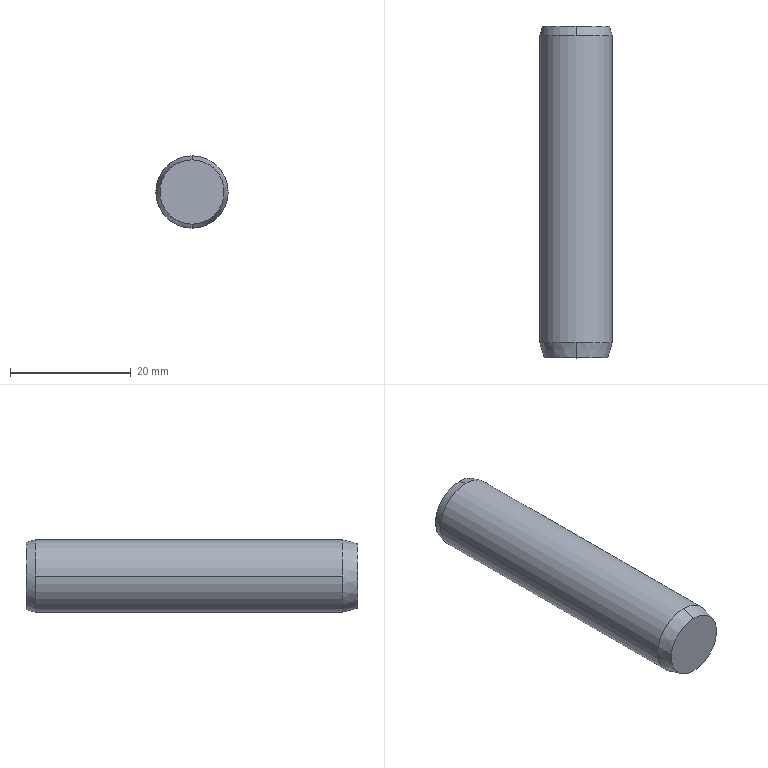Part | STEP file | 1 solid | 16 faces | box 12 x 55 x 12 mm | volume 5770 mm3 | cone 8 | cylinder 6 | plane 2 | commonest cylinder face diameters 4.917 x2 6.4 x2 12 x2
STEP:
#1=CARTESIAN_POINT('',(0.,-55.,5.33));
#2=VERTEX_POINT('',#1);
#3=CARTESIAN_POINT('',(0.,-55.,-5.33));
#4=VERTEX_POINT('',#3);
#5=CARTESIAN_POINT('',(0.,-55.,0.));
#6=DIRECTION('',(0.,1.,0.));
#7=DIRECTION('',(0.,0.,1.));
#8=AXIS2_PLACEMENT_3D('',#5,#6,#7);
#9=CIRCLE('',#8,5.33);
#10=EDGE_CURVE('',#2,#4,#9,.T.);
#11=ORIENTED_EDGE('',*,*,#10,.T.);
#12=CARTESIAN_POINT('',(0.,-52.5,-6.));
#13=VERTEX_POINT('',#12);
#14=CARTESIAN_POINT('',(0.,-55.,-5.33));
#15=DIRECTION('',(0.,0.9659,-0.2588));
#16=VECTOR('',#15,1000.);
#17=LINE('',#14,#16);
#18=EDGE_CURVE('',#4,#13,#17,.T.);
#19=ORIENTED_EDGE('',*,*,#18,.T.);
#20=CARTESIAN_POINT('',(6.,-52.5,0.));
#21=VERTEX_POINT('',#20);
#22=CARTESIAN_POINT('',(0.,-52.5,0.));
#23=DIRECTION('',(0.,1.,0.));
#24=DIRECTION('',(0.,0.,1.));
#25=AXIS2_PLACEMENT_3D('',#22,#23,#24);
#26=CIRCLE('',#25,6.);
#27=EDGE_CURVE('',#21,#13,#26,.T.);
#28=ORIENTED_EDGE('',*,*,#27,.F.);
#29=CARTESIAN_POINT('',(0.,-52.5,6.));
#30=VERTEX_POINT('',#29);
#31=CARTESIAN_POINT('',(0.,-52.5,0.));
#32=DIRECTION('',(0.,1.,0.));
#33=DIRECTION('',(0.,0.,1.));
#34=AXIS2_PLACEMENT_3D('',#31,#32,#33);
#35=CIRCLE('',#34,6.);
#36=EDGE_CURVE('',#30,#21,#35,.T.);
#37=ORIENTED_EDGE('',*,*,#36,.F.);
#38=CARTESIAN_POINT('',(0.,-55.,5.33));
#39=DIRECTION('',(0.,0.9659,0.2588));
#40=VECTOR('',#39,1000.);
#41=LINE('',#38,#40);
#42=EDGE_CURVE('',#2,#30,#41,.T.);
#43=ORIENTED_EDGE('',*,*,#42,.F.);
#44=EDGE_LOOP('',(#11,#19,#28,#37,#43));
#45=FACE_OUTER_BOUND('',#44,.T.);
#46=CARTESIAN_POINT('',(0.,-55.,0.));
#47=DIRECTION('',(0.,1.,0.));
#48=DIRECTION('',(0.,0.,1.));
#49=AXIS2_PLACEMENT_3D('',#46,#47,#48);
#50=CONICAL_SURFACE('',#49,5.33,0.2618);
#51=ADVANCED_FACE('',(#45),#50,.T.);
#52=CARTESIAN_POINT('',(-6.,-52.5,0.));
#53=VERTEX_POINT('',#52);
#54=CARTESIAN_POINT('',(0.,-52.5,0.));
#55=DIRECTION('',(0.,1.,0.));
#56=DIRECTION('',(0.,0.,1.));
#57=AXIS2_PLACEMENT_3D('',#54,#55,#56);
#58=CIRCLE('',#57,6.);
#59=EDGE_CURVE('',#53,#30,#58,.T.);
#60=ORIENTED_EDGE('',*,*,#59,.T.);
#61=ORIENTED_EDGE('',*,*,#36,.T.);
#62=CARTESIAN_POINT('',(6.,-1.6,0.));
#63=VERTEX_POINT('',#62);
#64=CARTESIAN_POINT('',(6.,-21.42,0.));
#65=DIRECTION('',(0.,1.,0.));
#66=VECTOR('',#65,1000.);
#67=LINE('',#64,#66);
#68=EDGE_CURVE('',#21,#63,#67,.T.);
#69=ORIENTED_EDGE('',*,*,#68,.T.);
#70=CARTESIAN_POINT('',(0.,-1.6,6.));
#71=VERTEX_POINT('',#70);
#72=CARTESIAN_POINT('',(0.,-1.6,0.));
#73=DIRECTION('',(0.,1.,0.));
#74=DIRECTION('',(0.,0.,1.));
#75=AXIS2_PLACEMENT_3D('',#72,#73,#74);
#76=CIRCLE('',#75,6.);
#77=EDGE_CURVE('',#71,#63,#76,.T.);
#78=ORIENTED_EDGE('',*,*,#77,.F.);
#79=CARTESIAN_POINT('',(-6.,-1.6,0.));
#80=VERTEX_POINT('',#79);
#81=CARTESIAN_POINT('',(0.,-1.6,0.));
#82=DIRECTION('',(0.,1.,0.));
#83=DIRECTION('',(0.,0.,1.));
#84=AXIS2_PLACEMENT_3D('',#81,#82,#83);
#85=CIRCLE('',#84,6.);
#86=EDGE_CURVE('',#80,#71,#85,.T.);
#87=ORIENTED_EDGE('',*,*,#86,.F.);
#88=CARTESIAN_POINT('',(-6.,-21.42,0.));
#89=DIRECTION('',(0.,1.,0.));
#90=VECTOR('',#89,1000.);
#91=LINE('',#88,#90);
#92=EDGE_CURVE('',#53,#80,#91,.T.);
#93=ORIENTED_EDGE('',*,*,#92,.F.);
#94=EDGE_LOOP('',(#60,#61,#69,#78,#87,#93));
#95=FACE_OUTER_BOUND('',#94,.T.);
#96=CARTESIAN_POINT('',(0.,-21.42,0.));
#97=DIRECTION('',(0.,1.,0.));
#98=DIRECTION('',(-1.,0.,0.));
#99=AXIS2_PLACEMENT_3D('',#96,#97,#98);
#100=CYLINDRICAL_SURFACE('',#99,6.);
#101=ADVANCED_FACE('',(#95),#100,.T.);
#102=CARTESIAN_POINT('',(0.,0.,5.571));
#103=VERTEX_POINT('',#102);
#104=CARTESIAN_POINT('',(0.,0.,-5.571));
#105=VERTEX_POINT('',#104);
#106=CARTESIAN_POINT('',(0.,0.,0.));
#107=DIRECTION('',(0.,1.,0.));
#108=DIRECTION('',(0.,0.,1.));
#109=AXIS2_PLACEMENT_3D('',#106,#107,#108);
#110=CIRCLE('',#109,5.571);
#111=EDGE_CURVE('',#103,#105,#110,.T.);
#112=ORIENTED_EDGE('',*,*,#111,.F.);
#113=CARTESIAN_POINT('',(0.,-1.6,6.));
#114=DIRECTION('',(0.,-0.9659,0.2588));
#115=VECTOR('',#114,1000.);
#116=LINE('',#113,#115);
#117=EDGE_CURVE('',#103,#71,#116,.T.);
#118=ORIENTED_EDGE('',*,*,#117,.T.);
#119=ORIENTED_EDGE('',*,*,#77,.T.);
#120=CARTESIAN_POINT('',(0.,-1.6,-6.));
#121=VERTEX_POINT('',#120);
#122=CARTESIAN_POINT('',(0.,-1.6,0.));
#123=DIRECTION('',(0.,1.,0.));
#124=DIRECTION('',(0.,0.,1.));
#125=AXIS2_PLACEMENT_3D('',#122,#123,#124);
#126=CIRCLE('',#125,6.);
#127=EDGE_CURVE('',#63,#121,#126,.T.);
#128=ORIENTED_EDGE('',*,*,#127,.T.);
#129=CARTESIAN_POINT('',(0.,-1.6,-6.));
#130=DIRECTION('',(0.,-0.9659,-0.2588));
#131=VECTOR('',#130,1000.);
#132=LINE('',#129,#131);
#133=EDGE_CURVE('',#105,#121,#132,.T.);
#134=ORIENTED_EDGE('',*,*,#133,.F.);
#135=EDGE_LOOP('',(#112,#118,#119,#128,#134));
#136=FACE_OUTER_BOUND('',#135,.T.);
#137=CARTESIAN_POINT('',(0.,-1.6,0.));
#138=DIRECTION('',(0.,-1.,0.));
#139=DIRECTION('',(0.,0.,-1.));
#140=AXIS2_PLACEMENT_3D('',#137,#138,#139);
#141=CONICAL_SURFACE('',#140,6.,0.2618);
#142=ADVANCED_FACE('',(#136),#141,.T.);
#143=CARTESIAN_POINT('',(0.,-21.42,0.));
#144=VERTEX_POINT('',#143);
#145=CARTESIAN_POINT('',(-2.459,-20.,0.));
#146=VERTEX_POINT('',#145);
#147=CARTESIAN_POINT('',(-2.459,-20.,0.));
#148=DIRECTION('',(-0.866,0.5,0.));
#149=VECTOR('',#148,1000.);
#150=LINE('',#147,#149);
#151=EDGE_CURVE('',#144,#146,#150,.T.);
#152=ORIENTED_EDGE('',*,*,#151,.F.);
#153=CARTESIAN_POINT('',(2.459,-20.,0.));
#154=VERTEX_POINT('',#153);
#155=CARTESIAN_POINT('',(2.459,-20.,0.));
#156=DIRECTION('',(0.866,0.5,0.));
#157=VECTOR('',#156,1000.);
#158=LINE('',#155,#157);
#159=EDGE_CURVE('',#144,#154,#158,.T.);
#160=ORIENTED_EDGE('',*,*,#159,.T.);
#161=CARTESIAN_POINT('',(0.,-20.,0.));
#162=DIRECTION('',(0.,1.,0.));
#163=DIRECTION('',(-1.,0.,0.));
#164=AXIS2_PLACEMENT_3D('',#161,#162,#163);
#165=CIRCLE('',#164,2.459);
#166=EDGE_CURVE('',#154,#146,#165,.T.);
#167=ORIENTED_EDGE('',*,*,#166,.T.);
#168=EDGE_LOOP('',(#152,#160,#167));
#169=FACE_OUTER_BOUND('',#168,.T.);
#170=CARTESIAN_POINT('',(0.,-20.,0.));
#171=DIRECTION('',(0.,1.,0.));
#172=DIRECTION('',(-1.,0.,0.));
#173=AXIS2_PLACEMENT_3D('',#170,#171,#172);
#174=CONICAL_SURFACE('',#173,2.459,1.047);
#175=ADVANCED_FACE('',(#169),#174,.F.);
#176=ORIENTED_EDGE('',*,*,#166,.F.);
#177=CARTESIAN_POINT('',(2.459,-1.628,0.));
#178=VERTEX_POINT('',#177);
#179=CARTESIAN_POINT('',(2.459,-21.42,0.));
#180=DIRECTION('',(0.,1.,0.));
#181=VECTOR('',#180,1000.);
#182=LINE('',#179,#181);
#183=EDGE_CURVE('',#154,#178,#182,.T.);
#184=ORIENTED_EDGE('',*,*,#183,.T.);
#185=CARTESIAN_POINT('',(-2.459,-1.628,0.));
#186=VERTEX_POINT('',#185);
#187=CARTESIAN_POINT('',(0.,-1.628,0.));
#188=DIRECTION('',(0.,1.,0.));
#189=DIRECTION('',(-1.,0.,0.));
#190=AXIS2_PLACEMENT_3D('',#187,#188,#189);
#191=CIRCLE('',#190,2.459);
#192=EDGE_CURVE('',#178,#186,#191,.T.);
#193=ORIENTED_EDGE('',*,*,#192,.T.);
#194=CARTESIAN_POINT('',(-2.459,-21.42,0.));
#195=DIRECTION('',(0.,1.,0.));
#196=VECTOR('',#195,1000.);
#197=LINE('',#194,#196);
#198=EDGE_CURVE('',#146,#186,#197,.T.);
#199=ORIENTED_EDGE('',*,*,#198,.F.);
#200=EDGE_LOOP('',(#176,#184,#193,#199));
#201=FACE_OUTER_BOUND('',#200,.T.);
#202=CARTESIAN_POINT('',(0.,-21.42,0.));
#203=DIRECTION('',(0.,1.,0.));
#204=DIRECTION('',(-1.,0.,0.));
#205=AXIS2_PLACEMENT_3D('',#202,#203,#204);
#206=CYLINDRICAL_SURFACE('',#205,2.459);
#207=ADVANCED_FACE('',(#201),#206,.F.);
#208=ORIENTED_EDGE('',*,*,#192,.F.);
#209=CARTESIAN_POINT('',(3.2,-1.2,0.));
#210=VERTEX_POINT('',#209);
#211=CARTESIAN_POINT('',(3.2,-1.2,0.));
#212=DIRECTION('',(0.866,0.5,0.));
#213=VECTOR('',#212,1000.);
#214=LINE('',#211,#213);
#215=EDGE_CURVE('',#178,#210,#214,.T.);
#216=ORIENTED_EDGE('',*,*,#215,.T.);
#217=CARTESIAN_POINT('',(-3.2,-1.2,0.));
#218=VERTEX_POINT('',#217);
#219=CARTESIAN_POINT('',(0.,-1.2,0.));
#220=DIRECTION('',(0.,1.,0.));
#221=DIRECTION('',(-1.,0.,0.));
#222=AXIS2_PLACEMENT_3D('',#219,#220,#221);
#223=CIRCLE('',#222,3.2);
#224=EDGE_CURVE('',#210,#218,#223,.T.);
#225=ORIENTED_EDGE('',*,*,#224,.T.);
#226=CARTESIAN_POINT('',(-3.2,-1.2,0.));
#227=DIRECTION('',(-0.866,0.5,0.));
#228=VECTOR('',#227,1000.);
#229=LINE('',#226,#228);
#230=EDGE_CURVE('',#186,#218,#229,.T.);
#231=ORIENTED_EDGE('',*,*,#230,.F.);
#232=EDGE_LOOP('',(#208,#216,#225,#231));
#233=FACE_OUTER_BOUND('',#232,.T.);
#234=CARTESIAN_POINT('',(0.,-1.2,0.));
#235=DIRECTION('',(0.,1.,0.));
#236=DIRECTION('',(-1.,0.,0.));
#237=AXIS2_PLACEMENT_3D('',#234,#235,#236);
#238=CONICAL_SURFACE('',#237,3.2,1.047);
#239=ADVANCED_FACE('',(#233),#238,.F.);
#240=ORIENTED_EDGE('',*,*,#224,.F.);
#241=CARTESIAN_POINT('',(3.2,0.,0.));
#242=VERTEX_POINT('',#241);
#243=CARTESIAN_POINT('',(3.2,-21.42,0.));
#244=DIRECTION('',(0.,1.,0.));
#245=VECTOR('',#244,1000.);
#246=LINE('',#243,#245);
#247=EDGE_CURVE('',#210,#242,#246,.T.);
#248=ORIENTED_EDGE('',*,*,#247,.T.);
#249=CARTESIAN_POINT('',(-3.2,0.,0.));
#250=VERTEX_POINT('',#249);
#251=CARTESIAN_POINT('',(0.,0.,0.));
#252=DIRECTION('',(0.,1.,0.));
#253=DIRECTION('',(-1.,0.,0.));
#254=AXIS2_PLACEMENT_3D('',#251,#252,#253);
#255=CIRCLE('',#254,3.2);
#256=EDGE_CURVE('',#242,#250,#255,.T.);
#257=ORIENTED_EDGE('',*,*,#256,.T.);
#258=CARTESIAN_POINT('',(-3.2,-21.42,0.));
#259=DIRECTION('',(0.,1.,0.));
#260=VECTOR('',#259,1000.);
#261=LINE('',#258,#260);
#262=EDGE_CURVE('',#218,#250,#261,.T.);
#263=ORIENTED_EDGE('',*,*,#262,.F.);
#264=EDGE_LOOP('',(#240,#248,#257,#263));
#265=FACE_OUTER_BOUND('',#264,.T.);
#266=CARTESIAN_POINT('',(0.,-21.42,0.));
#267=DIRECTION('',(0.,1.,0.));
#268=DIRECTION('',(-1.,0.,0.));
#269=AXIS2_PLACEMENT_3D('',#266,#267,#268);
#270=CYLINDRICAL_SURFACE('',#269,3.2);
#271=ADVANCED_FACE('',(#265),#270,.F.);
#272=CARTESIAN_POINT('',(0.,0.,0.));
#273=DIRECTION('',(0.,1.,0.));
#274=DIRECTION('',(-1.,0.,0.));
#275=AXIS2_PLACEMENT_3D('',#272,#273,#274);
#276=CIRCLE('',#275,3.2);
#277=EDGE_CURVE('',#250,#242,#276,.T.);
#278=ORIENTED_EDGE('',*,*,#277,.F.);
#279=ORIENTED_EDGE('',*,*,#256,.F.);
#280=EDGE_LOOP('',(#278,#279));
#281=FACE_BOUND('',#280,.T.);
#282=CARTESIAN_POINT('',(0.,0.,0.));
#283=DIRECTION('',(0.,1.,0.));
#284=DIRECTION('',(0.,0.,1.));
#285=AXIS2_PLACEMENT_3D('',#282,#283,#284);
#286=CIRCLE('',#285,5.571);
#287=EDGE_CURVE('',#105,#103,#286,.T.);
#288=ORIENTED_EDGE('',*,*,#287,.T.);
#289=ORIENTED_EDGE('',*,*,#111,.T.);
#290=EDGE_LOOP('',(#288,#289));
#291=FACE_OUTER_BOUND('',#290,.T.);
#292=CARTESIAN_POINT('',(6.,0.,0.));
#293=DIRECTION('',(0.,-1.,0.));
#294=DIRECTION('',(1.,0.,0.));
#295=AXIS2_PLACEMENT_3D('',#292,#293,#294);
#296=PLANE('',#295);
#297=ADVANCED_FACE('',(#281,#291),#296,.F.);
#298=ORIENTED_EDGE('',*,*,#247,.F.);
#299=CARTESIAN_POINT('',(0.,-1.2,0.));
#300=DIRECTION('',(0.,1.,0.));
#301=DIRECTION('',(-1.,0.,0.));
#302=AXIS2_PLACEMENT_3D('',#299,#300,#301);
#303=CIRCLE('',#302,3.2);
#304=EDGE_CURVE('',#218,#210,#303,.T.);
#305=ORIENTED_EDGE('',*,*,#304,.F.);
#306=ORIENTED_EDGE('',*,*,#262,.T.);
#307=ORIENTED_EDGE('',*,*,#277,.T.);
#308=EDGE_LOOP('',(#298,#305,#306,#307));
#309=FACE_OUTER_BOUND('',#308,.T.);
#310=CARTESIAN_POINT('',(0.,-21.42,0.));
#311=DIRECTION('',(0.,1.,0.));
#312=DIRECTION('',(-1.,0.,0.));
#313=AXIS2_PLACEMENT_3D('',#310,#311,#312);
#314=CYLINDRICAL_SURFACE('',#313,3.2);
#315=ADVANCED_FACE('',(#309),#314,.F.);
#316=ORIENTED_EDGE('',*,*,#215,.F.);
#317=CARTESIAN_POINT('',(0.,-1.628,0.));
#318=DIRECTION('',(0.,1.,0.));
#319=DIRECTION('',(-1.,0.,0.));
#320=AXIS2_PLACEMENT_3D('',#317,#318,#319);
#321=CIRCLE('',#320,2.459);
#322=EDGE_CURVE('',#186,#178,#321,.T.);
#323=ORIENTED_EDGE('',*,*,#322,.F.);
#324=ORIENTED_EDGE('',*,*,#230,.T.);
#325=ORIENTED_EDGE('',*,*,#304,.T.);
#326=EDGE_LOOP('',(#316,#323,#324,#325));
#327=FACE_OUTER_BOUND('',#326,.T.);
#328=CARTESIAN_POINT('',(0.,-1.2,0.));
#329=DIRECTION('',(0.,1.,0.));
#330=DIRECTION('',(-1.,0.,0.));
#331=AXIS2_PLACEMENT_3D('',#328,#329,#330);
#332=CONICAL_SURFACE('',#331,3.2,1.047);
#333=ADVANCED_FACE('',(#327),#332,.F.);
#334=ORIENTED_EDGE('',*,*,#183,.F.);
#335=CARTESIAN_POINT('',(0.,-20.,0.));
#336=DIRECTION('',(0.,1.,0.));
#337=DIRECTION('',(-1.,0.,0.));
#338=AXIS2_PLACEMENT_3D('',#335,#336,#337);
#339=CIRCLE('',#338,2.459);
#340=EDGE_CURVE('',#146,#154,#339,.T.);
#341=ORIENTED_EDGE('',*,*,#340,.F.);
#342=ORIENTED_EDGE('',*,*,#198,.T.);
#343=ORIENTED_EDGE('',*,*,#322,.T.);
#344=EDGE_LOOP('',(#334,#341,#342,#343));
#345=FACE_OUTER_BOUND('',#344,.T.);
#346=CARTESIAN_POINT('',(0.,-21.42,0.));
#347=DIRECTION('',(0.,1.,0.));
#348=DIRECTION('',(-1.,0.,0.));
#349=AXIS2_PLACEMENT_3D('',#346,#347,#348);
#350=CYLINDRICAL_SURFACE('',#349,2.459);
#351=ADVANCED_FACE('',(#345),#350,.F.);
#352=ORIENTED_EDGE('',*,*,#159,.F.);
#353=ORIENTED_EDGE('',*,*,#151,.T.);
#354=ORIENTED_EDGE('',*,*,#340,.T.);
#355=EDGE_LOOP('',(#352,#353,#354));
#356=FACE_OUTER_BOUND('',#355,.T.);
#357=CARTESIAN_POINT('',(0.,-20.,0.));
#358=DIRECTION('',(0.,1.,0.));
#359=DIRECTION('',(-1.,0.,0.));
#360=AXIS2_PLACEMENT_3D('',#357,#358,#359);
#361=CONICAL_SURFACE('',#360,2.459,1.047);
#362=ADVANCED_FACE('',(#356),#361,.F.);
#363=ORIENTED_EDGE('',*,*,#117,.F.);
#364=ORIENTED_EDGE('',*,*,#287,.F.);
#365=ORIENTED_EDGE('',*,*,#133,.T.);
#366=CARTESIAN_POINT('',(0.,-1.6,0.));
#367=DIRECTION('',(0.,1.,0.));
#368=DIRECTION('',(0.,0.,1.));
#369=AXIS2_PLACEMENT_3D('',#366,#367,#368);
#370=CIRCLE('',#369,6.);
#371=EDGE_CURVE('',#121,#80,#370,.T.);
#372=ORIENTED_EDGE('',*,*,#371,.T.);
#373=ORIENTED_EDGE('',*,*,#86,.T.);
#374=EDGE_LOOP('',(#363,#364,#365,#372,#373));
#375=FACE_OUTER_BOUND('',#374,.T.);
#376=CARTESIAN_POINT('',(0.,-1.6,0.));
#377=DIRECTION('',(0.,-1.,0.));
#378=DIRECTION('',(0.,0.,-1.));
#379=AXIS2_PLACEMENT_3D('',#376,#377,#378);
#380=CONICAL_SURFACE('',#379,6.,0.2618);
#381=ADVANCED_FACE('',(#375),#380,.T.);
#382=ORIENTED_EDGE('',*,*,#68,.F.);
#383=ORIENTED_EDGE('',*,*,#27,.T.);
#384=CARTESIAN_POINT('',(0.,-52.5,0.));
#385=DIRECTION('',(0.,1.,0.));
#386=DIRECTION('',(0.,0.,1.));
#387=AXIS2_PLACEMENT_3D('',#384,#385,#386);
#388=CIRCLE('',#387,6.);
#389=EDGE_CURVE('',#13,#53,#388,.T.);
#390=ORIENTED_EDGE('',*,*,#389,.T.);
#391=ORIENTED_EDGE('',*,*,#92,.T.);
#392=ORIENTED_EDGE('',*,*,#371,.F.);
#393=ORIENTED_EDGE('',*,*,#127,.F.);
#394=EDGE_LOOP('',(#382,#383,#390,#391,#392,#393));
#395=FACE_OUTER_BOUND('',#394,.T.);
#396=CARTESIAN_POINT('',(0.,-21.42,0.));
#397=DIRECTION('',(0.,1.,0.));
#398=DIRECTION('',(-1.,0.,0.));
#399=AXIS2_PLACEMENT_3D('',#396,#397,#398);
#400=CYLINDRICAL_SURFACE('',#399,6.);
#401=ADVANCED_FACE('',(#395),#400,.T.);
#402=ORIENTED_EDGE('',*,*,#18,.F.);
#403=CARTESIAN_POINT('',(0.,-55.,0.));
#404=DIRECTION('',(0.,1.,0.));
#405=DIRECTION('',(0.,0.,1.));
#406=AXIS2_PLACEMENT_3D('',#403,#404,#405);
#407=CIRCLE('',#406,5.33);
#408=EDGE_CURVE('',#4,#2,#407,.T.);
#409=ORIENTED_EDGE('',*,*,#408,.T.);
#410=ORIENTED_EDGE('',*,*,#42,.T.);
#411=ORIENTED_EDGE('',*,*,#59,.F.);
#412=ORIENTED_EDGE('',*,*,#389,.F.);
#413=EDGE_LOOP('',(#402,#409,#410,#411,#412));
#414=FACE_OUTER_BOUND('',#413,.T.);
#415=CARTESIAN_POINT('',(0.,-55.,0.));
#416=DIRECTION('',(0.,1.,0.));
#417=DIRECTION('',(0.,0.,1.));
#418=AXIS2_PLACEMENT_3D('',#415,#416,#417);
#419=CONICAL_SURFACE('',#418,5.33,0.2618);
#420=ADVANCED_FACE('',(#414),#419,.T.);
#421=ORIENTED_EDGE('',*,*,#10,.F.);
#422=ORIENTED_EDGE('',*,*,#408,.F.);
#423=EDGE_LOOP('',(#421,#422));
#424=FACE_OUTER_BOUND('',#423,.T.);
#425=CARTESIAN_POINT('',(0.,-55.,0.));
#426=DIRECTION('',(0.,1.,0.));
#427=DIRECTION('',(-1.,0.,0.));
#428=AXIS2_PLACEMENT_3D('',#425,#426,#427);
#429=PLANE('',#428);
#430=ADVANCED_FACE('',(#424),#429,.F.);
#431=CLOSED_SHELL('',(#51,#101,#142,#175,#207,#239,#271,#297,#315,#333,#351,#362,#381,#401,#420,#430));
#432=MANIFOLD_SOLID_BREP('',#431);
#433=CARTESIAN_POINT('',(0.,0.,0.));
#434=DIRECTION('',(0.,0.,1.));
#435=DIRECTION('',(1.,0.,0.));
#436=AXIS2_PLACEMENT_3D('',#433,#434,#435);
#437=(LENGTH_UNIT()NAMED_UNIT(*)SI_UNIT(.MILLI.,.METRE.));
#438=UNCERTAINTY_MEASURE_WITH_UNIT(LENGTH_MEASURE(0.00001),#437,'','');
#439=(NAMED_UNIT(*)PLANE_ANGLE_UNIT()SI_UNIT($,.RADIAN.));
#440=(NAMED_UNIT(*)SI_UNIT($,.STERADIAN.)SOLID_ANGLE_UNIT());
#441=(GEOMETRIC_REPRESENTATION_CONTEXT(3)GLOBAL_UNCERTAINTY_ASSIGNED_CONTEXT((#438))GLOBAL_UNIT_ASSIGNED_CONTEXT((#437,#439,#440))REPRESENTATION_CONTEXT('',''));
#442=ADVANCED_BREP_SHAPE_REPRESENTATION('',(#432,#436),#441);